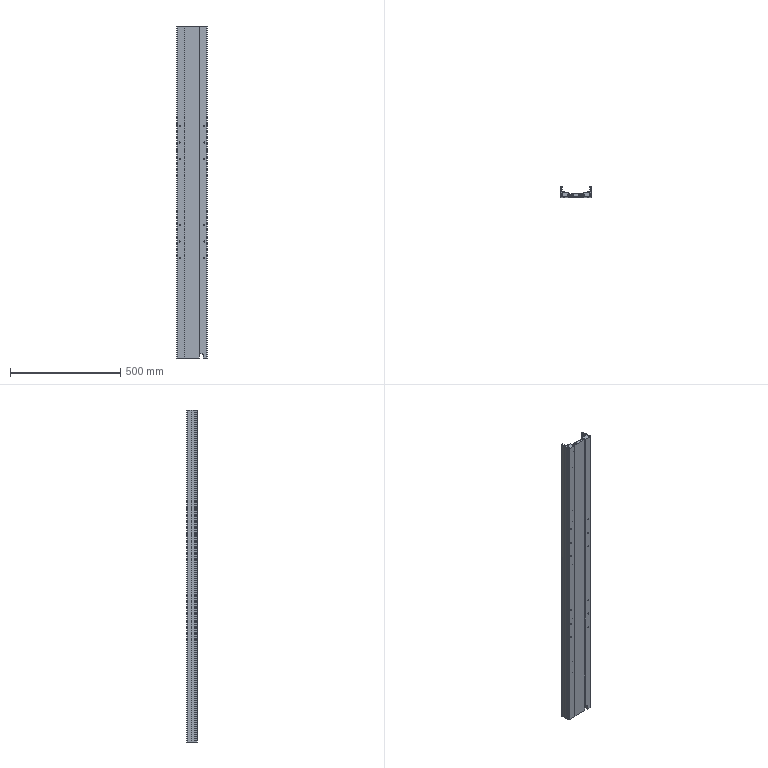Part | STEP file | SM140A-20-1140D-140A-600 Base SF600 | 1 solid | 369 faces | box 140 x 48 x 1508 mm | volume 3406004 mm3 | cylinder 203 | plane 166 | commonest cylinder face diameters 3.2 x102 10 x30 5.5 x24 4 x18 4.8 x16 2 x7